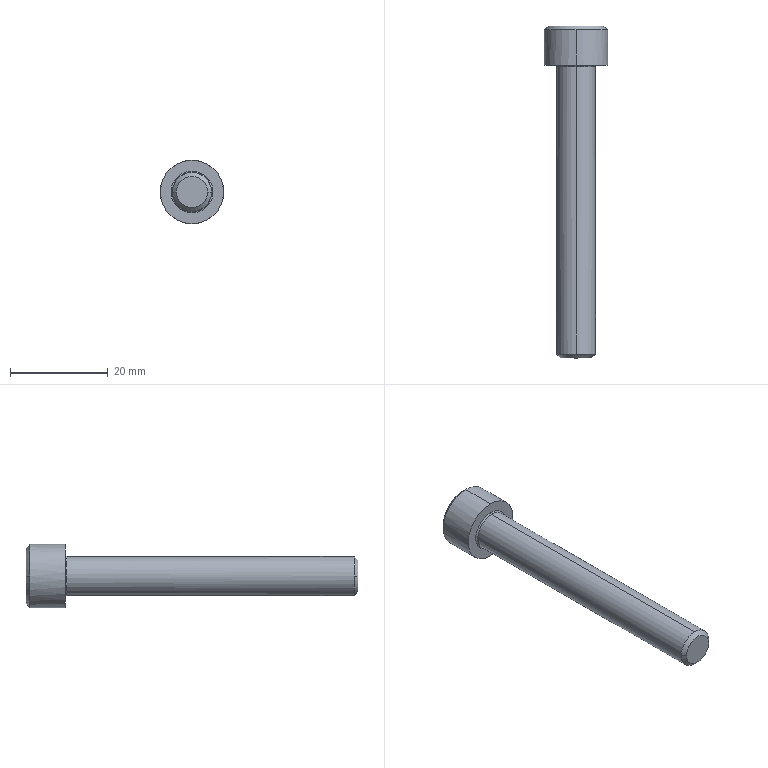Part | STEP file | 1 solid | 20 faces | box 13 x 68 x 13 mm | volume 3871 mm3 | plane 10 | cone 4 | cylinder 4 | spline 2 | commonest cylinder face diameters 8 x2 13 x2